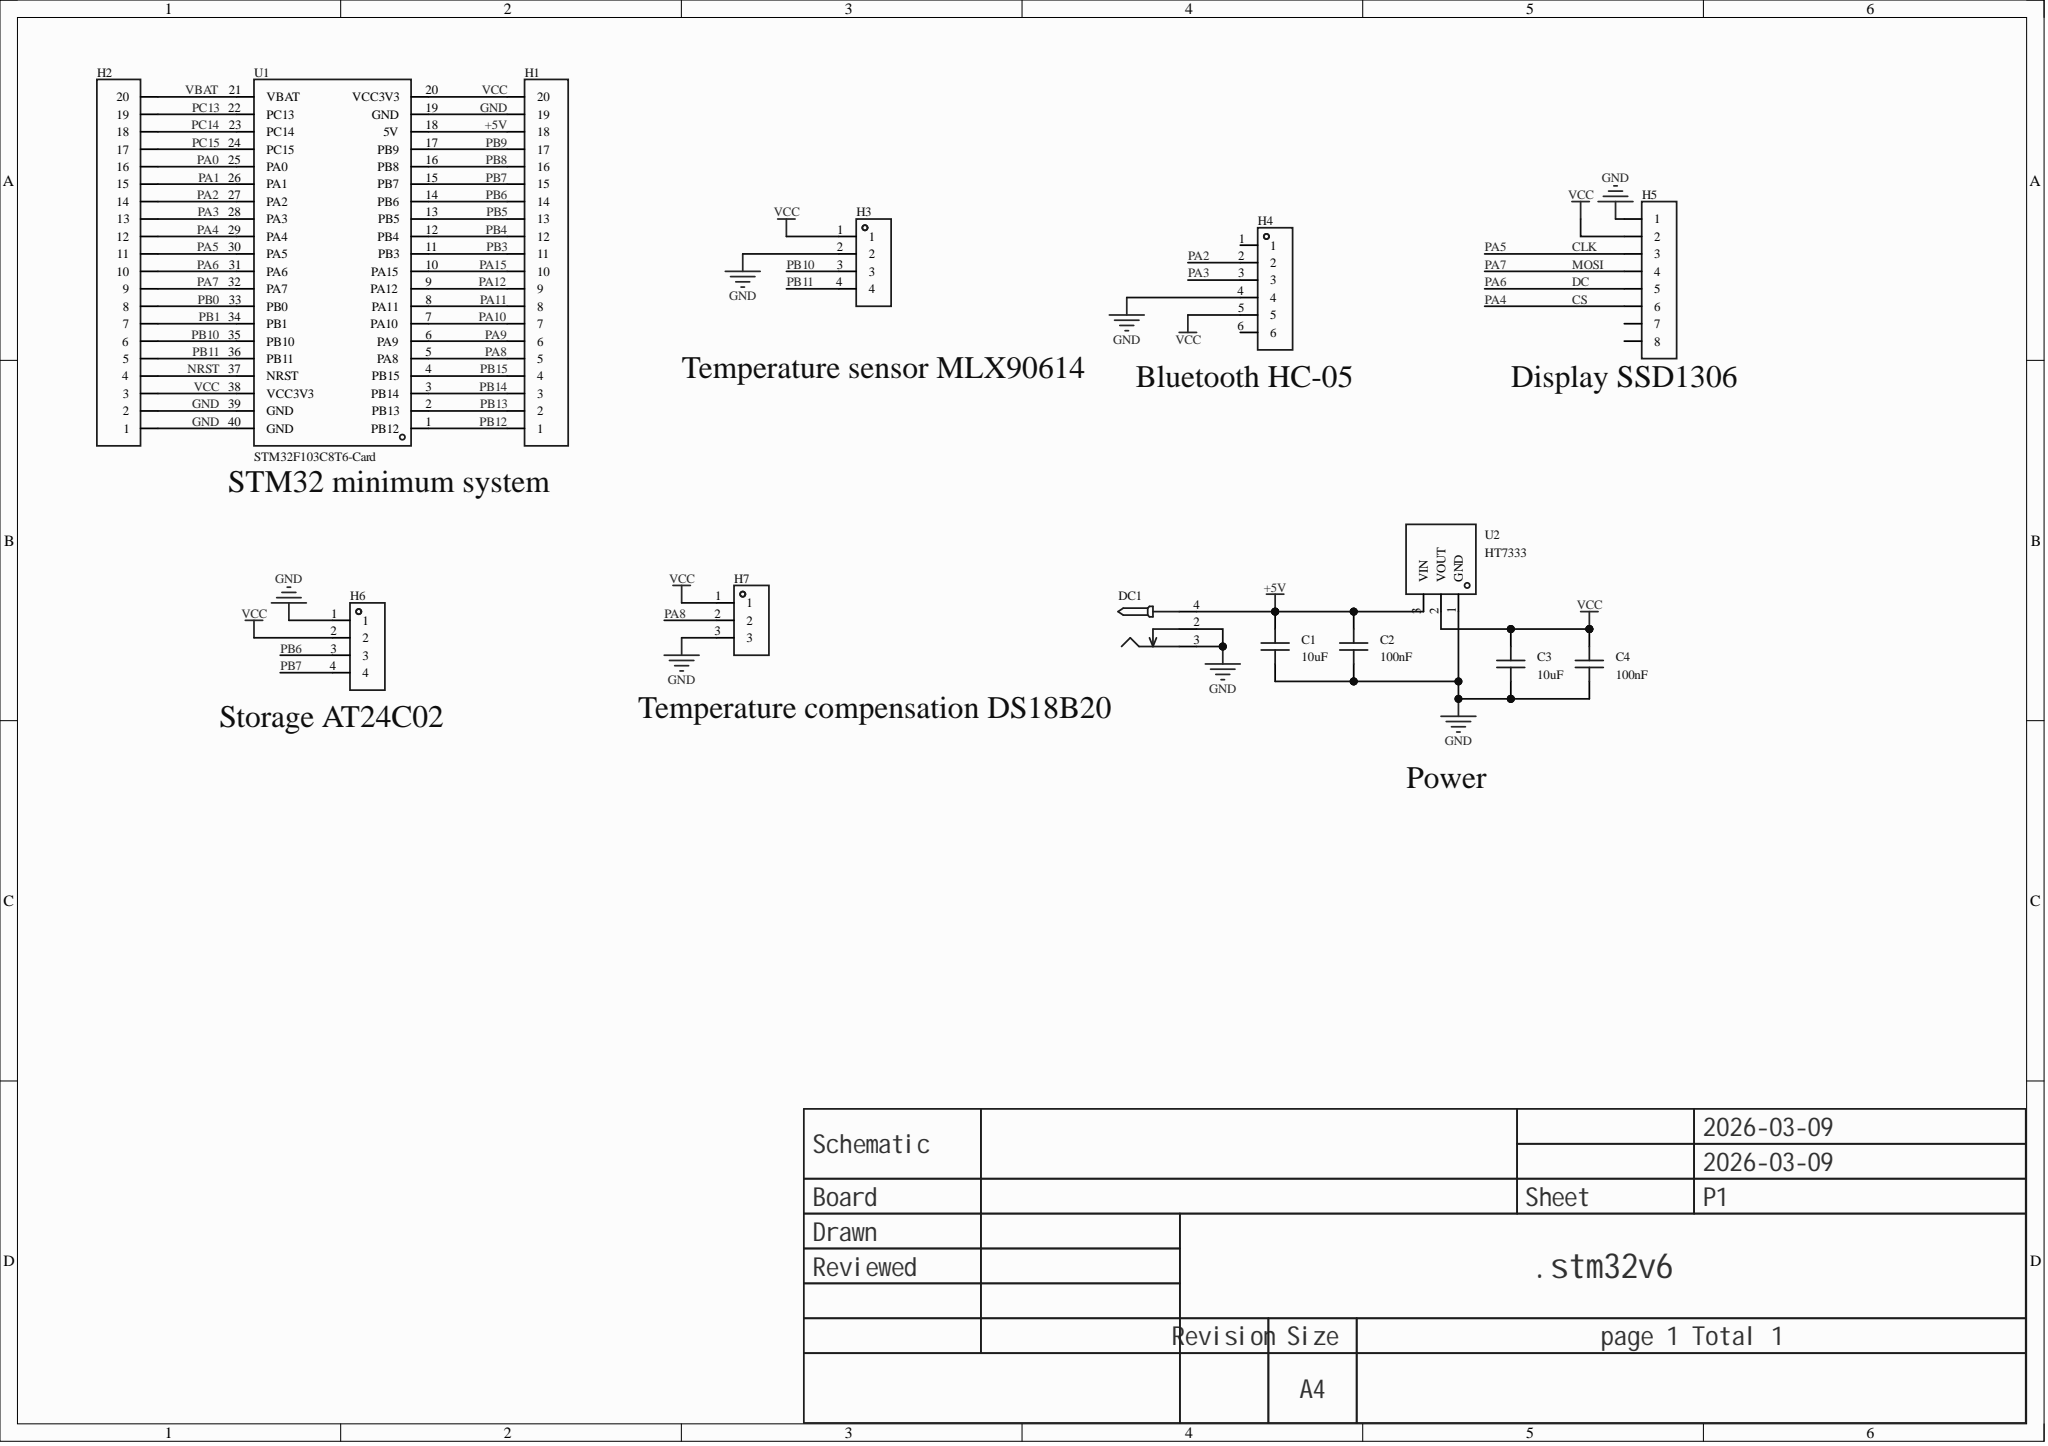Circuit board | Altium Designer | 14 parts | 37 nets
Bill of materials:
Comment,Description,Designator,Footprint,LibRef,Quantity
"10uF","","C1, C3","C0603","CAP_0603","2"
"100nF","","C2, C4","C0603","CAP_0603","2"
"","","DC1","DC-2.0","DC-005_2.0","1"
"","","H1, H2","HDR-TH_20P-P2.54-V-F","HDR-F_2.54_1x20P","2"
"","","H3, H6","HDR-TH_4P-P2.54-V-F","HDR-F_2.54_1x4P","2"
"","","H4","HDR-TH_6P-P2.54-V-F","HDR-F_2.54_1x6P","1"
"","","H5","HDR-TH_8P-P2.54-V-F-1","HDR-F_2.54_1x8P","1"
"","","H7","HDR-TH_3P-P2.54-V-F","HDR-F_2.54_1x3P","1"
"STM32F103C8T6-Card","","U1","CONN-TH_L53.3-W22.9_STM32F103C8T6-CARD","STM32F103C8T6-Card","1"
"HT7333","Output type: fixed; input voltage: 12V; output voltage: 3.3V; output current: 250mA; ripple rejection (PSRR): -; output polarity: positive;","U2","SOT-23-3_L2.9-W1.6-P1.90-LS2.8-BR","HT7333","1"
Netlist (Protel format):
[
C1
C0603
10uF



]
[
C2
C0603
100nF



]
[
C3
C0603
10uF



]
[
C4
C0603
100nF



]
[
DC1
DC-2.0




]
[
H1
HDR-TH_20P-P2.54-V-F




]
[
H2
HDR-TH_20P-P2.54-V-F




]
[
H3
HDR-TH_4P-P2.54-V-F




]
[
H4
HDR-TH_6P-P2.54-V-F




]
[
H5
HDR-TH_8P-P2.54-V-F-1




]
[
H6
HDR-TH_4P-P2.54-V-F




]
[
H7
HDR-TH_3P-P2.54-V-F




]
[
U1
CONN-TH_L53.3-W22.9_STM32F103C8T6-CARD
STM32F103C8T6-Card



]
[
U2
SOT-23-3_L2.9-W1.6-P1.90-LS2.8-BR
HT7333



]
(
VCC
C3-2
C4-2
H1-20
H2-3
H3-1
H4-5
H5-2
H6-2
H7-1
U1-20
U1-38
U2-2
)
(
VBAT
H2-20
U1-21
)
(
PC15
H2-17
U1-24
)
(
PC14
H2-18
U1-23
)
(
PC13
H2-19
U1-22
)
(
PB15
H1-4
U1-4
)
(
PB14
H1-3
U1-3
)
(
PB13
H1-2
U1-2
)
(
PB12
H1-1
U1-1
)
(
PB11
H2-5
H3-4
U1-36
)
(
PB10
H2-6
H3-3
U1-35
)
(
PB9
H1-17
U1-17
)
(
PB8
H1-16
U1-16
)
(
PB7
H1-15
H6-4
U1-15
)
(
PB6
H1-14
H6-3
U1-14
)
(
PB5
H1-13
U1-13
)
(
PB4
H1-12
U1-12
)
(
PB3
H1-11
U1-11
)
(
PB1
H2-7
U1-34
)
(
PB0
H2-8
U1-33
)
(
PA15
H1-10
U1-10
)
(
PA12
H1-9
U1-9
)
(
PA11
H1-8
U1-8
)
(
PA10
H1-7
U1-7
)
(
PA9
H1-6
U1-6
)
(
PA8
H1-5
H7-2
U1-5
)
(
PA3
H2-13
H4-3
U1-28
)
(
PA2
H2-14
H4-2
U1-27
)
(
PA1
H2-15
U1-26
)
(
PA0
H2-16
U1-25
)
(
NRST
H2-4
U1-37
)
(
MOSI
H2-9
H5-4
U1-32
)
(
GND
C1-1
C2-1
C3-1
C4-1
DC1-2
DC1-3
H1-19
H2-1
H2-2
H3-2
H4-4
H5-1
H6-1
H7-3
U1-19
U1-39
U1-40
U2-1
)
(
DC
H2-10
H5-5
U1-31
)
(
CS
H2-12
H5-6
U1-29
)
(
CLK
H2-11
H5-3
U1-30
)
(
+5V
C1-2
C2-2
DC1-4
H1-18
U1-18
U2-3
)